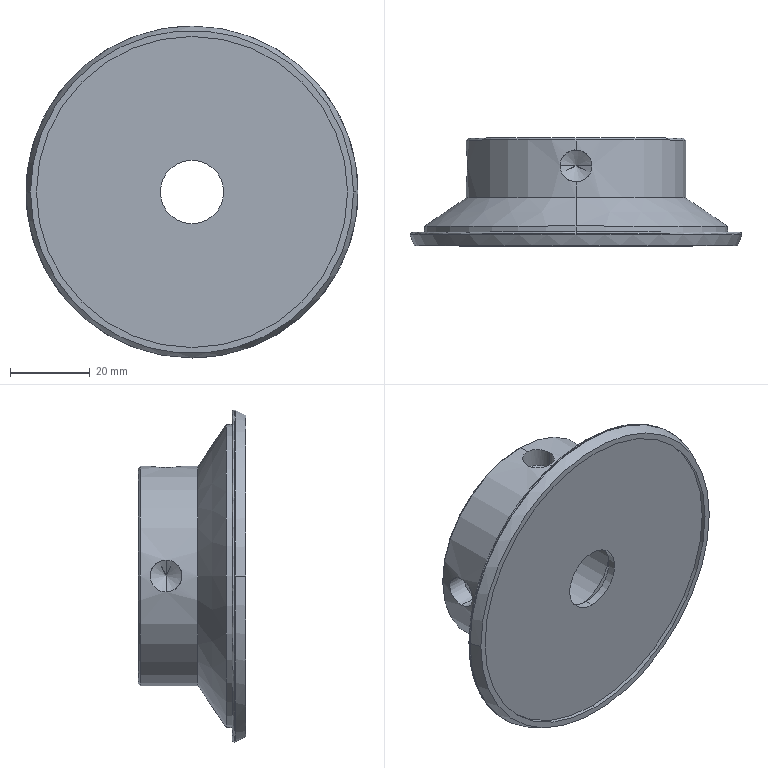Part | SolidWorks | features BaseBody 1 | 1 solid | 41 faces | box 83.227 x 27 x 83.227 mm | volume 68079 mm3 | cylinder 18 | cone 12 | plane 7 | spline 4 | commonest cylinder face diameters 8 x4 25 x4 15.9 x2 22 x2 55 x2 76 x2
STEP:
#1=CARTESIAN_POINT('',(0.,1.9,41.613));
#2=VERTEX_POINT('',#1);
#3=CARTESIAN_POINT('',(0.,1.9,-41.613));
#4=VERTEX_POINT('',#3);
#5=CARTESIAN_POINT('',(0.,1.9,0.));
#6=DIRECTION('',(0.,-1.,0.));
#7=DIRECTION('',(0.,0.,-1.));
#8=AXIS2_PLACEMENT_3D('',#5,#6,#7);
#9=CIRCLE('',#8,41.613);
#10=EDGE_CURVE('',#2,#4,#9,.T.);
#11=ORIENTED_EDGE('',*,*,#10,.F.);
#12=CARTESIAN_POINT('',(0.,2.4,41.113));
#13=VERTEX_POINT('',#12);
#14=CARTESIAN_POINT('',(0.,1.9,41.113));
#15=DIRECTION('',(-1.,0.,0.));
#16=DIRECTION('',(0.,0.,1.));
#17=AXIS2_PLACEMENT_3D('',#14,#15,#16);
#18=CIRCLE('',#17,0.5);
#19=EDGE_CURVE('',#2,#13,#18,.T.);
#20=ORIENTED_EDGE('',*,*,#19,.T.);
#21=CARTESIAN_POINT('',(0.,2.4,-41.113));
#22=VERTEX_POINT('',#21);
#23=CARTESIAN_POINT('',(0.,2.4,41.113));
#24=CARTESIAN_POINT('',(-82.227,2.4,41.113));
#25=CARTESIAN_POINT('',(-82.227,2.4,-41.113));
#26=CARTESIAN_POINT('',(0.,2.4,-41.113));
#27=(BOUNDED_CURVE()B_SPLINE_CURVE(3,(#23,#24,#25,#26),.UNSPECIFIED.,.F.,.F.)B_SPLINE_CURVE_WITH_KNOTS((4,4),(0.,1.),.UNSPECIFIED.)CURVE()GEOMETRIC_REPRESENTATION_ITEM()RATIONAL_B_SPLINE_CURVE((1.,0.3333,0.3333,1.))REPRESENTATION_ITEM(''));
#28=EDGE_CURVE('',#13,#22,#27,.T.);
#29=ORIENTED_EDGE('',*,*,#28,.T.);
#30=CARTESIAN_POINT('',(0.,1.9,-41.113));
#31=DIRECTION('',(1.,0.,0.));
#32=DIRECTION('',(0.,0.,-1.));
#33=AXIS2_PLACEMENT_3D('',#30,#31,#32);
#34=CIRCLE('',#33,0.5);
#35=EDGE_CURVE('',#4,#22,#34,.T.);
#36=ORIENTED_EDGE('',*,*,#35,.F.);
#37=EDGE_LOOP('',(#11,#20,#29,#36));
#38=FACE_OUTER_BOUND('',#37,.T.);
#39=CARTESIAN_POINT('',(0.,1.9,41.613));
#40=CARTESIAN_POINT('',(-83.227,1.9,41.613));
#41=CARTESIAN_POINT('',(-83.227,1.9,-41.613));
#42=CARTESIAN_POINT('',(0.,1.9,-41.613));
#43=CARTESIAN_POINT('',(0.,2.193,41.613));
#44=CARTESIAN_POINT('',(-83.227,2.193,41.613));
#45=CARTESIAN_POINT('',(-83.227,2.193,-41.613));
#46=CARTESIAN_POINT('',(0.,2.193,-41.613));
#47=CARTESIAN_POINT('',(0.,2.4,41.406));
#48=CARTESIAN_POINT('',(-82.813,2.4,41.406));
#49=CARTESIAN_POINT('',(-82.813,2.4,-41.406));
#50=CARTESIAN_POINT('',(0.,2.4,-41.406));
#51=CARTESIAN_POINT('',(0.,2.4,41.113));
#52=CARTESIAN_POINT('',(-82.227,2.4,41.113));
#53=CARTESIAN_POINT('',(-82.227,2.4,-41.113));
#54=CARTESIAN_POINT('',(0.,2.4,-41.113));
#55=(BOUNDED_SURFACE()B_SPLINE_SURFACE(3,3,((#39,#40,#41,#42),(#43,#44,#45,#46),(#47,#48,#49,#50),(#51,#52,#53,#54)),.UNSPECIFIED.,.F.,.F.,.F.)B_SPLINE_SURFACE_WITH_KNOTS((4,4),(4,4),(0.,1.),(0.,1.),.UNSPECIFIED.)GEOMETRIC_REPRESENTATION_ITEM()RATIONAL_B_SPLINE_SURFACE(((1.,0.3333,0.3333,1.),(0.8047,0.2682,0.2682,0.8047),(0.8047,0.2682,0.2682,0.8047),(1.,0.3333,0.3333,1.)))REPRESENTATION_ITEM('')SURFACE());
#56=ADVANCED_FACE('',(#38),#55,.T.);
#57=CARTESIAN_POINT('',(0.,1.715,41.578));
#58=VERTEX_POINT('',#57);
#59=CARTESIAN_POINT('',(-41.578,1.715,0.));
#60=VERTEX_POINT('',#59);
#61=CARTESIAN_POINT('',(0.,1.715,0.));
#62=DIRECTION('',(0.,-1.,0.));
#63=DIRECTION('',(0.,0.,1.));
#64=AXIS2_PLACEMENT_3D('',#61,#62,#63);
#65=CIRCLE('',#64,41.578);
#66=EDGE_CURVE('',#58,#60,#65,.T.);
#67=ORIENTED_EDGE('',*,*,#66,.F.);
#68=CARTESIAN_POINT('',(0.,1.9,41.113));
#69=DIRECTION('',(-1.,0.,0.));
#70=DIRECTION('',(0.,0.,1.));
#71=AXIS2_PLACEMENT_3D('',#68,#69,#70);
#72=CIRCLE('',#71,0.5);
#73=EDGE_CURVE('',#58,#2,#72,.T.);
#74=ORIENTED_EDGE('',*,*,#73,.T.);
#75=ORIENTED_EDGE('',*,*,#10,.T.);
#76=CARTESIAN_POINT('',(0.,1.715,-41.578));
#77=VERTEX_POINT('',#76);
#78=CARTESIAN_POINT('',(0.,1.9,-41.113));
#79=DIRECTION('',(1.,0.,0.));
#80=DIRECTION('',(0.,0.,-1.));
#81=AXIS2_PLACEMENT_3D('',#78,#79,#80);
#82=CIRCLE('',#81,0.5);
#83=EDGE_CURVE('',#77,#4,#82,.T.);
#84=ORIENTED_EDGE('',*,*,#83,.F.);
#85=CARTESIAN_POINT('',(0.,1.715,0.));
#86=DIRECTION('',(0.,-1.,0.));
#87=DIRECTION('',(0.,0.,1.));
#88=AXIS2_PLACEMENT_3D('',#85,#86,#87);
#89=CIRCLE('',#88,41.578);
#90=EDGE_CURVE('',#60,#77,#89,.T.);
#91=ORIENTED_EDGE('',*,*,#90,.F.);
#92=EDGE_LOOP('',(#67,#74,#75,#84,#91));
#93=FACE_OUTER_BOUND('',#92,.T.);
#94=CARTESIAN_POINT('',(0.,1.715,41.578));
#95=CARTESIAN_POINT('',(-83.156,1.715,41.578));
#96=CARTESIAN_POINT('',(-83.156,1.715,-41.578));
#97=CARTESIAN_POINT('',(0.,1.715,-41.578));
#98=CARTESIAN_POINT('',(0.,1.774,41.602));
#99=CARTESIAN_POINT('',(-83.203,1.774,41.602));
#100=CARTESIAN_POINT('',(-83.203,1.774,-41.602));
#101=CARTESIAN_POINT('',(0.,1.774,-41.602));
#102=CARTESIAN_POINT('',(0.,1.837,41.613));
#103=CARTESIAN_POINT('',(-83.227,1.837,41.613));
#104=CARTESIAN_POINT('',(-83.227,1.837,-41.613));
#105=CARTESIAN_POINT('',(0.,1.837,-41.613));
#106=CARTESIAN_POINT('',(0.,1.9,41.613));
#107=CARTESIAN_POINT('',(-83.227,1.9,41.613));
#108=CARTESIAN_POINT('',(-83.227,1.9,-41.613));
#109=CARTESIAN_POINT('',(0.,1.9,-41.613));
#110=(BOUNDED_SURFACE()B_SPLINE_SURFACE(3,3,((#94,#95,#96,#97),(#98,#99,#100,#101),(#102,#103,#104,#105),(#106,#107,#108,#109)),.UNSPECIFIED.,.F.,.F.,.F.)B_SPLINE_SURFACE_WITH_KNOTS((4,4),(4,4),(0.,1.),(0.,1.),.UNSPECIFIED.)GEOMETRIC_REPRESENTATION_ITEM()RATIONAL_B_SPLINE_SURFACE(((1.,0.3333,0.3333,1.),(0.9881,0.3294,0.3294,0.9881),(0.9881,0.3294,0.3294,0.9881),(1.,0.3333,0.3333,1.)))REPRESENTATION_ITEM('')SURFACE());
#111=ADVANCED_FACE('',(#93),#110,.T.);
#112=CARTESIAN_POINT('',(0.,0.,-39.));
#113=VERTEX_POINT('',#112);
#114=CARTESIAN_POINT('',(0.,0.,39.));
#115=VERTEX_POINT('',#114);
#116=CARTESIAN_POINT('',(0.,0.,0.));
#117=DIRECTION('',(0.,1.,0.));
#118=DIRECTION('',(0.,0.,-1.));
#119=AXIS2_PLACEMENT_3D('',#116,#117,#118);
#120=CIRCLE('',#119,39.);
#121=EDGE_CURVE('',#113,#115,#120,.T.);
#122=ORIENTED_EDGE('',*,*,#121,.T.);
#123=CARTESIAN_POINT('',(0.,-1.,39.));
#124=VERTEX_POINT('',#123);
#125=CARTESIAN_POINT('',(0.,0.,39.));
#126=DIRECTION('',(0.,-1.,0.));
#127=VECTOR('',#126,1000.);
#128=LINE('',#125,#127);
#129=EDGE_CURVE('',#115,#124,#128,.T.);
#130=ORIENTED_EDGE('',*,*,#129,.T.);
#131=CARTESIAN_POINT('',(0.,-1.,-39.));
#132=VERTEX_POINT('',#131);
#133=CARTESIAN_POINT('',(0.,-1.,0.));
#134=DIRECTION('',(0.,1.,0.));
#135=DIRECTION('',(0.,0.,-1.));
#136=AXIS2_PLACEMENT_3D('',#133,#134,#135);
#137=CIRCLE('',#136,39.);
#138=EDGE_CURVE('',#132,#124,#137,.T.);
#139=ORIENTED_EDGE('',*,*,#138,.F.);
#140=CARTESIAN_POINT('',(0.,0.,-39.));
#141=DIRECTION('',(0.,-1.,0.));
#142=VECTOR('',#141,1000.);
#143=LINE('',#140,#142);
#144=EDGE_CURVE('',#113,#132,#143,.T.);
#145=ORIENTED_EDGE('',*,*,#144,.F.);
#146=EDGE_LOOP('',(#122,#130,#139,#145));
#147=FACE_OUTER_BOUND('',#146,.T.);
#148=CARTESIAN_POINT('',(0.,0.,0.));
#149=DIRECTION('',(0.,-1.,0.));
#150=DIRECTION('',(0.,0.,-1.));
#151=AXIS2_PLACEMENT_3D('',#148,#149,#150);
#152=CYLINDRICAL_SURFACE('',#151,39.);
#153=ADVANCED_FACE('',(#147),#152,.F.);
#154=CARTESIAN_POINT('',(0.,2.,7.95));
#155=VERTEX_POINT('',#154);
#156=CARTESIAN_POINT('',(0.,2.,-7.95));
#157=VERTEX_POINT('',#156);
#158=CARTESIAN_POINT('',(0.,2.,0.));
#159=DIRECTION('',(0.,-1.,0.));
#160=DIRECTION('',(0.,0.,-1.));
#161=AXIS2_PLACEMENT_3D('',#158,#159,#160);
#162=CIRCLE('',#161,7.95);
#163=EDGE_CURVE('',#155,#157,#162,.T.);
#164=ORIENTED_EDGE('',*,*,#163,.F.);
#165=CARTESIAN_POINT('',(0.,0.,7.95));
#166=VERTEX_POINT('',#165);
#167=CARTESIAN_POINT('',(0.,0.,7.95));
#168=DIRECTION('',(0.,-1.,0.));
#169=VECTOR('',#168,1000.);
#170=LINE('',#167,#169);
#171=EDGE_CURVE('',#155,#166,#170,.T.);
#172=ORIENTED_EDGE('',*,*,#171,.T.);
#173=CARTESIAN_POINT('',(0.,0.,-7.95));
#174=VERTEX_POINT('',#173);
#175=CARTESIAN_POINT('',(0.,0.,0.));
#176=DIRECTION('',(0.,-1.,0.));
#177=DIRECTION('',(0.,0.,-1.));
#178=AXIS2_PLACEMENT_3D('',#175,#176,#177);
#179=CIRCLE('',#178,7.95);
#180=EDGE_CURVE('',#166,#174,#179,.T.);
#181=ORIENTED_EDGE('',*,*,#180,.T.);
#182=CARTESIAN_POINT('',(0.,0.,-7.95));
#183=DIRECTION('',(0.,-1.,0.));
#184=VECTOR('',#183,1000.);
#185=LINE('',#182,#184);
#186=EDGE_CURVE('',#157,#174,#185,.T.);
#187=ORIENTED_EDGE('',*,*,#186,.F.);
#188=EDGE_LOOP('',(#164,#172,#181,#187));
#189=FACE_OUTER_BOUND('',#188,.T.);
#190=CARTESIAN_POINT('',(0.,0.,0.));
#191=DIRECTION('',(0.,-1.,0.));
#192=DIRECTION('',(0.,0.,-1.));
#193=AXIS2_PLACEMENT_3D('',#190,#191,#192);
#194=CYLINDRICAL_SURFACE('',#193,7.95);
#195=ADVANCED_FACE('',(#189),#194,.F.);
#196=CARTESIAN_POINT('',(-40.5,-1.,0.));
#197=VERTEX_POINT('',#196);
#198=CARTESIAN_POINT('',(40.5,-1.,0.));
#199=VERTEX_POINT('',#198);
#200=CARTESIAN_POINT('',(0.,-1.,0.));
#201=DIRECTION('',(0.,1.,0.));
#202=DIRECTION('',(-1.,0.,0.));
#203=AXIS2_PLACEMENT_3D('',#200,#201,#202);
#204=CIRCLE('',#203,40.5);
#205=EDGE_CURVE('',#197,#199,#204,.T.);
#206=ORIENTED_EDGE('',*,*,#205,.T.);
#207=CARTESIAN_POINT('',(41.578,1.715,0.));
#208=VERTEX_POINT('',#207);
#209=CARTESIAN_POINT('',(41.578,1.715,0.));
#210=DIRECTION('',(0.369,0.9294,0.));
#211=VECTOR('',#210,1000.);
#212=LINE('',#209,#211);
#213=EDGE_CURVE('',#199,#208,#212,.T.);
#214=ORIENTED_EDGE('',*,*,#213,.T.);
#215=CARTESIAN_POINT('',(0.,1.715,0.));
#216=DIRECTION('',(0.,-1.,0.));
#217=DIRECTION('',(0.,0.,1.));
#218=AXIS2_PLACEMENT_3D('',#215,#216,#217);
#219=CIRCLE('',#218,41.578);
#220=EDGE_CURVE('',#208,#58,#219,.T.);
#221=ORIENTED_EDGE('',*,*,#220,.T.);
#222=ORIENTED_EDGE('',*,*,#66,.T.);
#223=CARTESIAN_POINT('',(-41.578,1.715,0.));
#224=DIRECTION('',(-0.369,0.9294,0.));
#225=VECTOR('',#224,1000.);
#226=LINE('',#223,#225);
#227=EDGE_CURVE('',#197,#60,#226,.T.);
#228=ORIENTED_EDGE('',*,*,#227,.F.);
#229=EDGE_LOOP('',(#206,#214,#221,#222,#228));
#230=FACE_OUTER_BOUND('',#229,.T.);
#231=CARTESIAN_POINT('',(0.,1.715,0.));
#232=DIRECTION('',(0.,1.,0.));
#233=DIRECTION('',(-1.,0.,0.));
#234=AXIS2_PLACEMENT_3D('',#231,#232,#233);
#235=CONICAL_SURFACE('',#234,41.578,0.378);
#236=ADVANCED_FACE('',(#230),#235,.T.);
#237=CARTESIAN_POINT('',(0.,5.,12.5));
#238=VERTEX_POINT('',#237);
#239=CARTESIAN_POINT('',(0.,5.,-12.5));
#240=VERTEX_POINT('',#239);
#241=CARTESIAN_POINT('',(0.,5.,0.));
#242=DIRECTION('',(0.,-1.,0.));
#243=DIRECTION('',(0.,0.,-1.));
#244=AXIS2_PLACEMENT_3D('',#241,#242,#243);
#245=CIRCLE('',#244,12.5);
#246=EDGE_CURVE('',#238,#240,#245,.T.);
#247=ORIENTED_EDGE('',*,*,#246,.F.);
#248=CARTESIAN_POINT('',(0.,2.,12.5));
#249=VERTEX_POINT('',#248);
#250=CARTESIAN_POINT('',(0.,0.,12.5));
#251=DIRECTION('',(0.,-1.,0.));
#252=VECTOR('',#251,1000.);
#253=LINE('',#250,#252);
#254=EDGE_CURVE('',#238,#249,#253,.T.);
#255=ORIENTED_EDGE('',*,*,#254,.T.);
#256=CARTESIAN_POINT('',(0.,2.,-12.5));
#257=VERTEX_POINT('',#256);
#258=CARTESIAN_POINT('',(0.,2.,0.));
#259=DIRECTION('',(0.,-1.,0.));
#260=DIRECTION('',(0.,0.,-1.));
#261=AXIS2_PLACEMENT_3D('',#258,#259,#260);
#262=CIRCLE('',#261,12.5);
#263=EDGE_CURVE('',#249,#257,#262,.T.);
#264=ORIENTED_EDGE('',*,*,#263,.T.);
#265=CARTESIAN_POINT('',(0.,0.,-12.5));
#266=DIRECTION('',(0.,-1.,0.));
#267=VECTOR('',#266,1000.);
#268=LINE('',#265,#267);
#269=EDGE_CURVE('',#240,#257,#268,.T.);
#270=ORIENTED_EDGE('',*,*,#269,.F.);
#271=EDGE_LOOP('',(#247,#255,#264,#270));
#272=FACE_OUTER_BOUND('',#271,.T.);
#273=CARTESIAN_POINT('',(0.,0.,0.));
#274=DIRECTION('',(0.,-1.,0.));
#275=DIRECTION('',(0.,0.,-1.));
#276=AXIS2_PLACEMENT_3D('',#273,#274,#275);
#277=CYLINDRICAL_SURFACE('',#276,12.5);
#278=ADVANCED_FACE('',(#272),#277,.F.);
#279=ORIENTED_EDGE('',*,*,#73,.F.);
#280=ORIENTED_EDGE('',*,*,#220,.F.);
#281=CARTESIAN_POINT('',(0.,1.715,0.));
#282=DIRECTION('',(0.,-1.,0.));
#283=DIRECTION('',(0.,0.,1.));
#284=AXIS2_PLACEMENT_3D('',#281,#282,#283);
#285=CIRCLE('',#284,41.578);
#286=EDGE_CURVE('',#77,#208,#285,.T.);
#287=ORIENTED_EDGE('',*,*,#286,.F.);
#288=ORIENTED_EDGE('',*,*,#83,.T.);
#289=CARTESIAN_POINT('',(0.,1.9,0.));
#290=DIRECTION('',(0.,-1.,0.));
#291=DIRECTION('',(0.,0.,-1.));
#292=AXIS2_PLACEMENT_3D('',#289,#290,#291);
#293=CIRCLE('',#292,41.613);
#294=EDGE_CURVE('',#4,#2,#293,.T.);
#295=ORIENTED_EDGE('',*,*,#294,.T.);
#296=EDGE_LOOP('',(#279,#280,#287,#288,#295));
#297=FACE_OUTER_BOUND('',#296,.T.);
#298=CARTESIAN_POINT('',(0.,1.715,-41.578));
#299=CARTESIAN_POINT('',(83.156,1.715,-41.578));
#300=CARTESIAN_POINT('',(83.156,1.715,41.578));
#301=CARTESIAN_POINT('',(0.,1.715,41.578));
#302=CARTESIAN_POINT('',(0.,1.774,-41.602));
#303=CARTESIAN_POINT('',(83.203,1.774,-41.602));
#304=CARTESIAN_POINT('',(83.203,1.774,41.602));
#305=CARTESIAN_POINT('',(0.,1.774,41.602));
#306=CARTESIAN_POINT('',(0.,1.837,-41.613));
#307=CARTESIAN_POINT('',(83.227,1.837,-41.613));
#308=CARTESIAN_POINT('',(83.227,1.837,41.613));
#309=CARTESIAN_POINT('',(0.,1.837,41.613));
#310=CARTESIAN_POINT('',(0.,1.9,-41.613));
#311=CARTESIAN_POINT('',(83.227,1.9,-41.613));
#312=CARTESIAN_POINT('',(83.227,1.9,41.613));
#313=CARTESIAN_POINT('',(0.,1.9,41.613));
#314=(BOUNDED_SURFACE()B_SPLINE_SURFACE(3,3,((#298,#299,#300,#301),(#302,#303,#304,#305),(#306,#307,#308,#309),(#310,#311,#312,#313)),.UNSPECIFIED.,.F.,.F.,.F.)B_SPLINE_SURFACE_WITH_KNOTS((4,4),(4,4),(0.,1.),(0.,1.),.UNSPECIFIED.)GEOMETRIC_REPRESENTATION_ITEM()RATIONAL_B_SPLINE_SURFACE(((1.,0.3333,0.3333,1.),(0.9881,0.3294,0.3294,0.9881),(0.9881,0.3294,0.3294,0.9881),(1.,0.3333,0.3333,1.)))REPRESENTATION_ITEM('')SURFACE());
#315=ADVANCED_FACE('',(#297),#314,.T.);
#316=CARTESIAN_POINT('',(0.,14.,11.));
#317=VERTEX_POINT('',#316);
#318=CARTESIAN_POINT('',(0.,14.,-11.));
#319=VERTEX_POINT('',#318);
#320=CARTESIAN_POINT('',(0.,14.,0.));
#321=DIRECTION('',(0.,-1.,0.));
#322=DIRECTION('',(0.,0.,-1.));
#323=AXIS2_PLACEMENT_3D('',#320,#321,#322);
#324=CIRCLE('',#323,11.);
#325=EDGE_CURVE('',#317,#319,#324,.T.);
#326=ORIENTED_EDGE('',*,*,#325,.F.);
#327=CARTESIAN_POINT('',(0.,5.,11.));
#328=VERTEX_POINT('',#327);
#329=CARTESIAN_POINT('',(0.,0.,11.));
#330=DIRECTION('',(0.,-1.,0.));
#331=VECTOR('',#330,1000.);
#332=LINE('',#329,#331);
#333=EDGE_CURVE('',#317,#328,#332,.T.);
#334=ORIENTED_EDGE('',*,*,#333,.T.);
#335=CARTESIAN_POINT('',(0.,5.,-11.));
#336=VERTEX_POINT('',#335);
#337=CARTESIAN_POINT('',(0.,5.,0.));
#338=DIRECTION('',(0.,-1.,0.));
#339=DIRECTION('',(0.,0.,-1.));
#340=AXIS2_PLACEMENT_3D('',#337,#338,#339);
#341=CIRCLE('',#340,11.);
#342=EDGE_CURVE('',#328,#336,#341,.T.);
#343=ORIENTED_EDGE('',*,*,#342,.T.);
#344=CARTESIAN_POINT('',(0.,0.,-11.));
#345=DIRECTION('',(0.,-1.,0.));
#346=VECTOR('',#345,1000.);
#347=LINE('',#344,#346);
#348=EDGE_CURVE('',#319,#336,#347,.T.);
#349=ORIENTED_EDGE('',*,*,#348,.F.);
#350=EDGE_LOOP('',(#326,#334,#343,#349));
#351=FACE_OUTER_BOUND('',#350,.T.);
#352=CARTESIAN_POINT('',(0.,0.,0.));
#353=DIRECTION('',(0.,-1.,0.));
#354=DIRECTION('',(0.,0.,-1.));
#355=AXIS2_PLACEMENT_3D('',#352,#353,#354);
#356=CYLINDRICAL_SURFACE('',#355,11.);
#357=ADVANCED_FACE('',(#351),#356,.F.);
#358=CARTESIAN_POINT('',(0.,3.9,-38.));
#359=VERTEX_POINT('',#358);
#360=CARTESIAN_POINT('',(0.,3.9,38.));
#361=VERTEX_POINT('',#360);
#362=CARTESIAN_POINT('',(0.,3.9,0.));
#363=DIRECTION('',(0.,-1.,0.));
#364=DIRECTION('',(0.,0.,-1.));
#365=AXIS2_PLACEMENT_3D('',#362,#363,#364);
#366=CIRCLE('',#365,38.);
#367=EDGE_CURVE('',#359,#361,#366,.T.);
#368=ORIENTED_EDGE('',*,*,#367,.T.);
#369=CARTESIAN_POINT('',(0.,2.4,38.));
#370=VERTEX_POINT('',#369);
#371=CARTESIAN_POINT('',(0.,0.,38.));
#372=DIRECTION('',(0.,-1.,0.));
#373=VECTOR('',#372,1000.);
#374=LINE('',#371,#373);
#375=EDGE_CURVE('',#361,#370,#374,.T.);
#376=ORIENTED_EDGE('',*,*,#375,.T.);
#377=CARTESIAN_POINT('',(0.,2.4,-38.));
#378=VERTEX_POINT('',#377);
#379=CARTESIAN_POINT('',(0.,2.4,0.));
#380=DIRECTION('',(0.,1.,0.));
#381=DIRECTION('',(0.,0.,-1.));
#382=AXIS2_PLACEMENT_3D('',#379,#380,#381);
#383=CIRCLE('',#382,38.);
#384=EDGE_CURVE('',#370,#378,#383,.T.);
#385=ORIENTED_EDGE('',*,*,#384,.T.);
#386=CARTESIAN_POINT('',(0.,0.,-38.));
#387=DIRECTION('',(0.,-1.,0.));
#388=VECTOR('',#387,1000.);
#389=LINE('',#386,#388);
#390=EDGE_CURVE('',#359,#378,#389,.T.);
#391=ORIENTED_EDGE('',*,*,#390,.F.);
#392=EDGE_LOOP('',(#368,#376,#385,#391));
#393=FACE_OUTER_BOUND('',#392,.T.);
#394=CARTESIAN_POINT('',(0.,0.,0.));
#395=DIRECTION('',(0.,-1.,0.));
#396=DIRECTION('',(0.,0.,-1.));
#397=AXIS2_PLACEMENT_3D('',#394,#395,#396);
#398=CYLINDRICAL_SURFACE('',#397,38.);
#399=ADVANCED_FACE('',(#393),#398,.T.);
#400=CARTESIAN_POINT('',(0.,11.,-27.5));
#401=VERTEX_POINT('',#400);
#402=CARTESIAN_POINT('',(0.,11.,27.5));
#403=VERTEX_POINT('',#402);
#404=CARTESIAN_POINT('',(0.,11.,0.));
#405=DIRECTION('',(0.,-1.,0.));
#406=DIRECTION('',(0.,0.,-1.));
#407=AXIS2_PLACEMENT_3D('',#404,#405,#406);
#408=CIRCLE('',#407,27.5);
#409=EDGE_CURVE('',#401,#403,#408,.T.);
#410=ORIENTED_EDGE('',*,*,#409,.T.);
#411=CARTESIAN_POINT('',(0.,3.9,38.));
#412=DIRECTION('',(0.,-0.5602,0.8284));
#413=VECTOR('',#412,1000.);
#414=LINE('',#411,#413);
#415=EDGE_CURVE('',#403,#361,#414,.T.);
#416=ORIENTED_EDGE('',*,*,#415,.T.);
#417=ORIENTED_EDGE('',*,*,#367,.F.);
#418=CARTESIAN_POINT('',(0.,3.9,-38.));
#419=DIRECTION('',(0.,-0.5602,-0.8284));
#420=VECTOR('',#419,1000.);
#421=LINE('',#418,#420);
#422=EDGE_CURVE('',#401,#359,#421,.T.);
#423=ORIENTED_EDGE('',*,*,#422,.F.);
#424=EDGE_LOOP('',(#410,#416,#417,#423));
#425=FACE_OUTER_BOUND('',#424,.T.);
#426=CARTESIAN_POINT('',(0.,3.9,0.));
#427=DIRECTION('',(0.,-1.,0.));
#428=DIRECTION('',(0.,0.,-1.));
#429=AXIS2_PLACEMENT_3D('',#426,#427,#428);
#430=CONICAL_SURFACE('',#429,38.,0.9762);
#431=ADVANCED_FACE('',(#425),#430,.T.);
#432=CARTESIAN_POINT('',(0.,25.5,12.5));
#433=VERTEX_POINT('',#432);
#434=CARTESIAN_POINT('',(0.,25.5,-12.5));
#435=VERTEX_POINT('',#434);
#436=CARTESIAN_POINT('',(0.,25.5,0.));
#437=DIRECTION('',(0.,-1.,0.));
#438=DIRECTION('',(0.,0.,-1.));
#439=AXIS2_PLACEMENT_3D('',#436,#437,#438);
#440=CIRCLE('',#439,12.5);
#441=EDGE_CURVE('',#433,#435,#440,.T.);
#442=ORIENTED_EDGE('',*,*,#441,.F.);
#443=CARTESIAN_POINT('',(0.,14.,12.5));
#444=VERTEX_POINT('',#443);
#445=CARTESIAN_POINT('',(0.,0.,12.5));
#446=DIRECTION('',(0.,-1.,0.));
#447=VECTOR('',#446,1000.);
#448=LINE('',#445,#447);
#449=EDGE_CURVE('',#433,#444,#448,.T.);
#450=ORIENTED_EDGE('',*,*,#449,.T.);
#451=CARTESIAN_POINT('',(0.,14.,-12.5));
#452=VERTEX_POINT('',#451);
#453=CARTESIAN_POINT('',(0.,14.,0.));
#454=DIRECTION('',(0.,-1.,0.));
#455=DIRECTION('',(0.,0.,-1.));
#456=AXIS2_PLACEMENT_3D('',#453,#454,#455);
#457=CIRCLE('',#456,12.5);
#458=EDGE_CURVE('',#444,#452,#457,.T.);
#459=ORIENTED_EDGE('',*,*,#458,.T.);
#460=CARTESIAN_POINT('',(0.,0.,-12.5));
#461=DIRECTION('',(0.,-1.,0.));
#462=VECTOR('',#461,1000.);
#463=LINE('',#460,#462);
#464=EDGE_CURVE('',#435,#452,#463,.T.);
#465=ORIENTED_EDGE('',*,*,#464,.F.);
#466=EDGE_LOOP('',(#442,#450,#459,#465));
#467=FACE_OUTER_BOUND('',#466,.T.);
#468=CARTESIAN_POINT('',(0.,0.,0.));
#469=DIRECTION('',(0.,-1.,0.));
#470=DIRECTION('',(0.,0.,-1.));
#471=AXIS2_PLACEMENT_3D('',#468,#469,#470);
#472=CYLINDRICAL_SURFACE('',#471,12.5);
#473=ADVANCED_FACE('',(#467),#472,.F.);
#474=CARTESIAN_POINT('',(27.5,25.5,0.));
#475=VERTEX_POINT('',#474);
#476=CARTESIAN_POINT('',(0.,25.5,27.5));
#477=VERTEX_POINT('',#476);
#478=CARTESIAN_POINT('',(0.,25.5,0.));
#479=DIRECTION('',(0.,-1.,0.));
#480=DIRECTION('',(0.,0.,-1.));
#481=AXIS2_PLACEMENT_3D('',#478,#479,#480);
#482=CIRCLE('',#481,27.5);
#483=EDGE_CURVE('',#475,#477,#482,.T.);
#484=ORIENTED_EDGE('',*,*,#483,.T.);
#485=CARTESIAN_POINT('',(0.,23.,27.5));
#486=VERTEX_POINT('',#485);
#487=CARTESIAN_POINT('',(0.,0.,27.5));
#488=DIRECTION('',(0.,-1.,0.));
#489=VECTOR('',#488,1000.);
#490=LINE('',#487,#489);
#491=EDGE_CURVE('',#477,#486,#490,.T.);
#492=ORIENTED_EDGE('',*,*,#491,.T.);
#493=CARTESIAN_POINT('',(4.,19.,27.208));
#494=VERTEX_POINT('',#493);
#495=CARTESIAN_POINT('',(0.,23.,27.5));
#496=CARTESIAN_POINT('',(0.2645,23.,27.5));
#497=CARTESIAN_POINT('',(0.5245,22.974,27.496));
#498=CARTESIAN_POINT('',(1.036,22.872,27.482));
#499=CARTESIAN_POINT('',(1.29,22.795,27.471));
#500=CARTESIAN_POINT('',(1.774,22.595,27.444));
#501=CARTESIAN_POINT('',(2.004,22.472,27.428));
#502=CARTESIAN_POINT('',(2.438,22.182,27.393));
#503=CARTESIAN_POINT('',(2.643,22.013,27.373));
#504=CARTESIAN_POINT('',(3.012,21.645,27.335));
#505=CARTESIAN_POINT('',(3.177,21.444,27.316));
#506=CARTESIAN_POINT('',(3.47,21.008,27.281));
#507=CARTESIAN_POINT('',(3.594,20.776,27.264));
#508=CARTESIAN_POINT('',(3.794,20.295,27.237));
#509=CARTESIAN_POINT('',(3.871,20.043,27.226));
#510=CARTESIAN_POINT('',(3.974,19.526,27.211));
#511=CARTESIAN_POINT('',(4.,19.264,27.208));
#512=CARTESIAN_POINT('',(4.,19.,27.208));
#513=B_SPLINE_CURVE_WITH_KNOTS('',3,(#495,#496,#497,#498,#499,#500,#501,#502,#503,#504,#505,#506,#507,#508,#509,#510,#511,#512),.UNSPECIFIED.,.F.,.F.,(4,2,2,2,2,2,2,2,4),(-0.006257,-0.005475,-0.004693,-0.003911,-0.003128,-0.002346,-0.001564,-0.0007821,0.),.UNSPECIFIED.);
#514=EDGE_CURVE('',#486,#494,#513,.T.);
#515=ORIENTED_EDGE('',*,*,#514,.T.);
#516=CARTESIAN_POINT('',(0.,15.,27.5));
#517=VERTEX_POINT('',#516);
#518=CARTESIAN_POINT('',(4.,19.,27.208));
#519=CARTESIAN_POINT('',(4.,18.736,27.208));
#520=CARTESIAN_POINT('',(3.974,18.476,27.211));
#521=CARTESIAN_POINT('',(3.872,17.964,27.226));
#522=CARTESIAN_POINT('',(3.795,17.71,27.237));
#523=CARTESIAN_POINT('',(3.595,17.226,27.264));
#524=CARTESIAN_POINT('',(3.472,16.996,27.28));
#525=CARTESIAN_POINT('',(3.182,16.562,27.316));
#526=CARTESIAN_POINT('',(3.013,16.357,27.335));
#527=CARTESIAN_POINT('',(2.645,15.988,27.373));
#528=CARTESIAN_POINT('',(2.444,15.823,27.392));
#529=CARTESIAN_POINT('',(2.008,15.53,27.427));
#530=CARTESIAN_POINT('',(1.776,15.406,27.444));
#531=CARTESIAN_POINT('',(1.295,15.206,27.471));
#532=CARTESIAN_POINT('',(1.043,15.129,27.481));
#533=CARTESIAN_POINT('',(0.526,15.026,27.496));
#534=CARTESIAN_POINT('',(0.2645,15.,27.5));
#535=CARTESIAN_POINT('',(0.,15.,27.5));
#536=B_SPLINE_CURVE_WITH_KNOTS('',3,(#518,#519,#520,#521,#522,#523,#524,#525,#526,#527,#528,#529,#530,#531,#532,#533,#534,#535),.UNSPECIFIED.,.F.,.F.,(4,2,2,2,2,2,2,2,4),(0.,0.0007821,0.001564,0.002346,0.003128,0.003911,0.004693,0.005475,0.006257),.UNSPECIFIED.);
#537=EDGE_CURVE('',#494,#517,#536,.T.);
#538=ORIENTED_EDGE('',*,*,#537,.T.);
#539=CARTESIAN_POINT('',(0.,0.,27.5));
#540=DIRECTION('',(0.,-1.,0.));
#541=VECTOR('',#540,1000.);
#542=LINE('',#539,#541);
#543=EDGE_CURVE('',#517,#403,#542,.T.);
#544=ORIENTED_EDGE('',*,*,#543,.T.);
#545=ORIENTED_EDGE('',*,*,#409,.F.);
#546=CARTESIAN_POINT('',(0.,25.5,-27.5));
#547=VERTEX_POINT('',#546);
#548=CARTESIAN_POINT('',(0.,0.,-27.5));
#549=DIRECTION('',(0.,-1.,0.));
#550=VECTOR('',#549,1000.);
#551=LINE('',#548,#550);
#552=EDGE_CURVE('',#547,#401,#551,.T.);
#553=ORIENTED_EDGE('',*,*,#552,.F.);
#554=CARTESIAN_POINT('',(0.,25.5,0.));
#555=DIRECTION('',(0.,-1.,0.));
#556=DIRECTION('',(0.,0.,-1.));
#557=AXIS2_PLACEMENT_3D('',#554,#555,#556);
#558=CIRCLE('',#557,27.5);
#559=EDGE_CURVE('',#547,#475,#558,.T.);
#560=ORIENTED_EDGE('',*,*,#559,.T.);
#561=EDGE_LOOP('',(#484,#492,#515,#538,#544,#545,#553,#560));
#562=FACE_OUTER_BOUND('',#561,.T.);
#563=CARTESIAN_POINT('',(0.,0.,0.));
#564=DIRECTION('',(0.,-1.,0.));
#565=DIRECTION('',(0.,0.,-1.));
#566=AXIS2_PLACEMENT_3D('',#563,#564,#565);
#567=CYLINDRICAL_SURFACE('',#566,27.5);
#568=ADVANCED_FACE('',(#562),#567,.T.);
#569=ORIENTED_EDGE('',*,*,#441,.T.);
#570=CARTESIAN_POINT('',(0.,26.,-13.));
#571=VERTEX_POINT('',#570);
#572=CARTESIAN_POINT('',(0.,26.,-13.));
#573=DIRECTION('',(0.,0.7071,-0.7071));
#574=VECTOR('',#573,1000.);
#575=LINE('',#572,#574);
#576=EDGE_CURVE('',#435,#571,#575,.T.);
#577=ORIENTED_EDGE('',*,*,#576,.T.);
#578=CARTESIAN_POINT('',(0.,26.,13.));
#579=VERTEX_POINT('',#578);
#580=CARTESIAN_POINT('',(0.,26.,0.));
#581=DIRECTION('',(0.,-1.,0.));
#582=DIRECTION('',(0.,0.,1.));
#583=AXIS2_PLACEMENT_3D('',#580,#581,#582);
#584=CIRCLE('',#583,13.);
#585=EDGE_CURVE('',#579,#571,#584,.T.);
#586=ORIENTED_EDGE('',*,*,#585,.F.);
#587=CARTESIAN_POINT('',(0.,26.,13.));
#588=DIRECTION('',(0.,0.7071,0.7071));
#589=VECTOR('',#588,1000.);
#590=LINE('',#587,#589);
#591=EDGE_CURVE('',#433,#579,#590,.T.);
#592=ORIENTED_EDGE('',*,*,#591,.F.);
#593=EDGE_LOOP('',(#569,#577,#586,#592));
#594=FACE_OUTER_BOUND('',#593,.T.);
#595=CARTESIAN_POINT('',(0.,26.,0.));
#596=DIRECTION('',(0.,1.,0.));
#597=DIRECTION('',(0.,0.,1.));
#598=AXIS2_PLACEMENT_3D('',#595,#596,#597);
#599=CONICAL_SURFACE('',#598,13.,0.7854);
#600=ADVANCED_FACE('',(#594),#599,.F.);
#601=CARTESIAN_POINT('',(-4.,19.,22.5));
#602=VERTEX_POINT('',#601);
#603=CARTESIAN_POINT('',(4.,19.,22.5));
#604=VERTEX_POINT('',#603);
#605=CARTESIAN_POINT('',(0.,19.,22.5));
#606=DIRECTION('',(0.,0.,1.));
#607=DIRECTION('',(1.,0.,0.));
#608=AXIS2_PLACEMENT_3D('',#605,#606,#607);
#609=CIRCLE('',#608,4.);
#610=EDGE_CURVE('',#602,#604,#609,.T.);
#611=ORIENTED_EDGE('',*,*,#610,.F.);
#612=CARTESIAN_POINT('',(-4.,19.,27.208));
#613=VERTEX_POINT('',#612);
#614=CARTESIAN_POINT('',(-4.,19.,27.5));
#615=DIRECTION('',(0.,0.,1.));
#616=VECTOR('',#615,1000.);
#617=LINE('',#614,#616);
#618=EDGE_CURVE('',#602,#613,#617,.T.);
#619=ORIENTED_EDGE('',*,*,#618,.T.);
#620=CARTESIAN_POINT('',(0.,15.,27.5));
#621=CARTESIAN_POINT('',(-0.2645,15.,27.5));
#622=CARTESIAN_POINT('',(-0.5245,15.026,27.496));
#623=CARTESIAN_POINT('',(-1.036,15.128,27.482));
#624=CARTESIAN_POINT('',(-1.29,15.205,27.471));
#625=CARTESIAN_POINT('',(-1.774,15.405,27.444));
#626=CARTESIAN_POINT('',(-2.004,15.528,27.428));
#627=CARTESIAN_POINT('',(-2.438,15.818,27.393));
#628=CARTESIAN_POINT('',(-2.643,15.987,27.373));
#629=CARTESIAN_POINT('',(-3.012,16.355,27.335));
#630=CARTESIAN_POINT('',(-3.177,16.556,27.316));
#631=CARTESIAN_POINT('',(-3.47,16.992,27.281));
#632=CARTESIAN_POINT('',(-3.594,17.224,27.264));
#633=CARTESIAN_POINT('',(-3.794,17.705,27.237));
#634=CARTESIAN_POINT('',(-3.871,17.957,27.226));
#635=CARTESIAN_POINT('',(-3.974,18.474,27.211));
#636=CARTESIAN_POINT('',(-4.,18.736,27.208));
#637=CARTESIAN_POINT('',(-4.,19.,27.208));
#638=B_SPLINE_CURVE_WITH_KNOTS('',3,(#620,#621,#622,#623,#624,#625,#626,#627,#628,#629,#630,#631,#632,#633,#634,#635,#636,#637),.UNSPECIFIED.,.F.,.F.,(4,2,2,2,2,2,2,2,4),(0.006257,0.007039,0.007821,0.008603,0.009385,0.01017,0.01095,0.01173,0.01251),.UNSPECIFIED.);
#639=EDGE_CURVE('',#517,#613,#638,.T.);
#640=ORIENTED_EDGE('',*,*,#639,.F.);
#641=ORIENTED_EDGE('',*,*,#537,.F.);
#642=CARTESIAN_POINT('',(4.,19.,27.5));
#643=DIRECTION('',(0.,0.,1.));
#644=VECTOR('',#643,1000.);
#645=LINE('',#642,#644);
#646=EDGE_CURVE('',#604,#494,#645,.T.);
#647=ORIENTED_EDGE('',*,*,#646,.F.);
#648=EDGE_LOOP('',(#611,#619,#640,#641,#647));
#649=FACE_OUTER_BOUND('',#648,.T.);
#650=CARTESIAN_POINT('',(0.,19.,27.5));
#651=DIRECTION('',(0.,0.,1.));
#652=DIRECTION('',(1.,0.,0.));
#653=AXIS2_PLACEMENT_3D('',#650,#651,#652);
#654=CYLINDRICAL_SURFACE('',#653,4.);
#655=ADVANCED_FACE('',(#649),#654,.F.);
#656=CARTESIAN_POINT('',(27.,26.,0.));
#657=VERTEX_POINT('',#656);
#658=CARTESIAN_POINT('',(-27.,26.,0.));
#659=VERTEX_POINT('',#658);
#660=CARTESIAN_POINT('',(0.,26.,0.));
#661=DIRECTION('',(0.,-1.,0.));
#662=DIRECTION('',(1.,0.,0.));
#663=AXIS2_PLACEMENT_3D('',#660,#661,#662);
#664=CIRCLE('',#663,27.);
#665=EDGE_CURVE('',#657,#659,#664,.T.);
#666=ORIENTED_EDGE('',*,*,#665,.T.);
#667=CARTESIAN_POINT('',(-27.5,25.5,0.));
#668=VERTEX_POINT('',#667);
#669=CARTESIAN_POINT('',(-27.5,25.5,0.));
#670=DIRECTION('',(-0.7071,-0.7071,0.));
#671=VECTOR('',#670,1000.);
#672=LINE('',#669,#671);
#673=EDGE_CURVE('',#659,#668,#672,.T.);
#674=ORIENTED_EDGE('',*,*,#673,.T.);
#675=CARTESIAN_POINT('',(0.,25.5,0.));
#676=DIRECTION('',(0.,-1.,0.));
#677=DIRECTION('',(0.,0.,-1.));
#678=AXIS2_PLACEMENT_3D('',#675,#676,#677);
#679=CIRCLE('',#678,27.5);
#680=EDGE_CURVE('',#477,#668,#679,.T.);
#681=ORIENTED_EDGE('',*,*,#680,.F.);
#682=ORIENTED_EDGE('',*,*,#483,.F.);
#683=CARTESIAN_POINT('',(27.5,25.5,0.));
#684=DIRECTION('',(0.7071,-0.7071,0.));
#685=VECTOR('',#684,1000.);
#686=LINE('',#683,#685);
#687=EDGE_CURVE('',#657,#475,#686,.T.);
#688=ORIENTED_EDGE('',*,*,#687,.F.);
#689=EDGE_LOOP('',(#666,#674,#681,#682,#688));
#690=FACE_OUTER_BOUND('',#689,.T.);
#691=CARTESIAN_POINT('',(0.,25.5,0.));
#692=DIRECTION('',(0.,-1.,0.));
#693=DIRECTION('',(1.,0.,0.));
#694=AXIS2_PLACEMENT_3D('',#691,#692,#693);
#695=CONICAL_SURFACE('',#694,27.5,0.7854);
#696=ADVANCED_FACE('',(#690),#695,.T.);
#697=CARTESIAN_POINT('',(-22.5,19.,-4.));
#698=VERTEX_POINT('',#697);
#699=CARTESIAN_POINT('',(-22.5,19.,4.));
#700=VERTEX_POINT('',#699);
#701=CARTESIAN_POINT('',(-22.5,19.,0.));
#702=DIRECTION('',(-1.,0.,0.));
#703=DIRECTION('',(0.,0.,1.));
#704=AXIS2_PLACEMENT_3D('',#701,#702,#703);
#705=CIRCLE('',#704,4.);
#706=EDGE_CURVE('',#698,#700,#705,.T.);
#707=ORIENTED_EDGE('',*,*,#706,.F.);
#708=CARTESIAN_POINT('',(-27.208,19.,-4.));
#709=VERTEX_POINT('',#708);
#710=CARTESIAN_POINT('',(-27.5,19.,-4.));
#711=DIRECTION('',(-1.,0.,0.));
#712=VECTOR('',#711,1000.);
#713=LINE('',#710,#712);
#714=EDGE_CURVE('',#698,#709,#713,.T.);
#715=ORIENTED_EDGE('',*,*,#714,.T.);
#716=CARTESIAN_POINT('',(-27.208,19.,4.));
#717=VERTEX_POINT('',#716);
#718=CARTESIAN_POINT('',(-27.208,19.,4.));
#719=CARTESIAN_POINT('',(-27.208,18.735,4.));
#720=CARTESIAN_POINT('',(-27.211,18.475,3.974));
#721=CARTESIAN_POINT('',(-27.226,17.964,3.872));
#722=CARTESIAN_POINT('',(-27.237,17.709,3.795));
#723=CARTESIAN_POINT('',(-27.264,17.225,3.594));
#724=CARTESIAN_POINT('',(-27.28,16.996,3.471));
#725=CARTESIAN_POINT('',(-27.316,16.561,3.181));
#726=CARTESIAN_POINT('',(-27.335,16.356,3.013));
#727=CARTESIAN_POINT('',(-27.373,15.987,2.644));
#728=CARTESIAN_POINT('',(-27.392,15.822,2.443));
#729=CARTESIAN_POINT('',(-27.428,15.529,2.006));
#730=CARTESIAN_POINT('',(-27.444,15.405,1.774));
#731=CARTESIAN_POINT('',(-27.471,15.206,1.293));
#732=CARTESIAN_POINT('',(-27.482,15.129,1.04));
#733=CARTESIAN_POINT('',(-27.496,15.026,0.5239));
#734=CARTESIAN_POINT('',(-27.5,15.,0.2642));
#735=CARTESIAN_POINT('',(-27.5,15.,-0.2582));
#736=CARTESIAN_POINT('',(-27.496,15.026,-0.5236));
#737=CARTESIAN_POINT('',(-27.482,15.128,-1.037));
#738=CARTESIAN_POINT('',(-27.471,15.203,-1.286));
#739=CARTESIAN_POINT('',(-27.444,15.404,-1.771));
#740=CARTESIAN_POINT('',(-27.428,15.529,-2.005));
#741=CARTESIAN_POINT('',(-27.393,15.818,-2.438));
#742=CARTESIAN_POINT('',(-27.374,15.984,-2.64));
#743=CARTESIAN_POINT('',(-27.335,16.356,-3.013));
#744=CARTESIAN_POINT('',(-27.316,16.558,-3.178));
#745=CARTESIAN_POINT('',(-27.281,16.99,-3.468));
#746=CARTESIAN_POINT('',(-27.264,17.224,-3.594));
#747=CARTESIAN_POINT('',(-27.237,17.708,-3.795));
#748=CARTESIAN_POINT('',(-27.226,17.957,-3.871));
#749=CARTESIAN_POINT('',(-27.211,18.471,-3.973));
#750=CARTESIAN_POINT('',(-27.208,18.735,-4.));
#751=CARTESIAN_POINT('',(-27.208,19.,-4.));
#752=B_SPLINE_CURVE_WITH_KNOTS('',3,(#718,#719,#720,#721,#722,#723,#724,#725,#726,#727,#728,#729,#730,#731,#732,#733,#734,#735,#736,#737,#738,#739,#740,#741,#742,#743,#744,#745,#746,#747,#748,#749,#750,#751),.UNSPECIFIED.,.F.,.F.,(4,2,2,2,2,2,2,2,2,2,2,2,2,2,2,2,4),(0.01252,0.0133,0.01408,0.01487,0.01565,0.01643,0.01721,0.018,0.01878,0.01956,0.02034,0.02113,0.02191,0.02269,0.02347,0.02426,0.02504),.UNSPECIFIED.);
#753=EDGE_CURVE('',#717,#709,#752,.T.);
#754=ORIENTED_EDGE('',*,*,#753,.F.);
#755=CARTESIAN_POINT('',(-27.5,19.,4.));
#756=DIRECTION('',(-1.,0.,0.));
#757=VECTOR('',#756,1000.);
#758=LINE('',#755,#757);
#759=EDGE_CURVE('',#700,#717,#758,.T.);
#760=ORIENTED_EDGE('',*,*,#759,.F.);
#761=EDGE_LOOP('',(#707,#715,#754,#760));
#762=FACE_OUTER_BOUND('',#761,.T.);
#763=CARTESIAN_POINT('',(-27.5,19.,0.));
#764=DIRECTION('',(-1.,0.,0.));
#765=DIRECTION('',(0.,0.,1.));
#766=AXIS2_PLACEMENT_3D('',#763,#764,#765);
#767=CYLINDRICAL_SURFACE('',#766,4.);
#768=ADVANCED_FACE('',(#762),#767,.F.);
#769=CARTESIAN_POINT('',(0.,19.,20.097));
#770=VERTEX_POINT('',#769);
#771=CARTESIAN_POINT('',(4.,19.,22.5));
#772=DIRECTION('',(0.8572,0.,0.515));
#773=VECTOR('',#772,1000.);
#774=LINE('',#771,#773);
#775=EDGE_CURVE('',#770,#604,#774,.T.);
#776=ORIENTED_EDGE('',*,*,#775,.F.);
#777=CARTESIAN_POINT('',(-4.,19.,22.5));
#778=DIRECTION('',(-0.8572,0.,0.515));
#779=VECTOR('',#778,1000.);
#780=LINE('',#777,#779);
#781=EDGE_CURVE('',#770,#602,#780,.T.);
#782=ORIENTED_EDGE('',*,*,#781,.T.);
#783=ORIENTED_EDGE('',*,*,#610,.T.);
#784=EDGE_LOOP('',(#776,#782,#783));
#785=FACE_OUTER_BOUND('',#784,.T.);
#786=CARTESIAN_POINT('',(0.,19.,22.5));
#787=DIRECTION('',(0.,0.,1.));
#788=DIRECTION('',(1.,0.,0.));
#789=AXIS2_PLACEMENT_3D('',#786,#787,#788);
#790=CONICAL_SURFACE('',#789,4.,1.03);
#791=ADVANCED_FACE('',(#785),#790,.F.);
#792=CARTESIAN_POINT('',(-20.097,19.,0.));
#793=VERTEX_POINT('',#792);
#794=CARTESIAN_POINT('',(-22.5,19.,4.));
#795=DIRECTION('',(-0.515,0.,0.8572));
#796=VECTOR('',#795,1000.);
#797=LINE('',#794,#796);
#798=EDGE_CURVE('',#793,#700,#797,.T.);
#799=ORIENTED_EDGE('',*,*,#798,.F.);
#800=CARTESIAN_POINT('',(-22.5,19.,-4.));
#801=DIRECTION('',(-0.515,0.,-0.8572));
#802=VECTOR('',#801,1000.);
#803=LINE('',#800,#802);
#804=EDGE_CURVE('',#793,#698,#803,.T.);
#805=ORIENTED_EDGE('',*,*,#804,.T.);
#806=ORIENTED_EDGE('',*,*,#706,.T.);
#807=EDGE_LOOP('',(#799,#805,#806));
#808=FACE_OUTER_BOUND('',#807,.T.);
#809=CARTESIAN_POINT('',(-22.5,19.,0.));
#810=DIRECTION('',(-1.,0.,0.));
#811=DIRECTION('',(0.,0.,1.));
#812=AXIS2_PLACEMENT_3D('',#809,#810,#811);
#813=CONICAL_SURFACE('',#812,4.,1.03);
#814=ADVANCED_FACE('',(#808),#813,.F.);
#815=ORIENTED_EDGE('',*,*,#121,.F.);
#816=CARTESIAN_POINT('',(0.,0.,0.));
#817=DIRECTION('',(0.,1.,0.));
#818=DIRECTION('',(0.,0.,-1.));
#819=AXIS2_PLACEMENT_3D('',#816,#817,#818);
#820=CIRCLE('',#819,39.);
#821=EDGE_CURVE('',#115,#113,#820,.T.);
#822=ORIENTED_EDGE('',*,*,#821,.F.);
#823=EDGE_LOOP('',(#815,#822));
#824=FACE_OUTER_BOUND('',#823,.T.);
#825=CARTESIAN_POINT('',(0.,0.,0.));
#826=DIRECTION('',(0.,-1.,0.));
#827=DIRECTION('',(0.,0.,-1.));
#828=AXIS2_PLACEMENT_3D('',#825,#826,#827);
#829=CIRCLE('',#828,7.95);
#830=EDGE_CURVE('',#174,#166,#829,.T.);
#831=ORIENTED_EDGE('',*,*,#830,.F.);
#832=ORIENTED_EDGE('',*,*,#180,.F.);
#833=EDGE_LOOP('',(#831,#832));
#834=FACE_BOUND('',#833,.T.);
#835=CARTESIAN_POINT('',(-7.95,0.,0.));
#836=DIRECTION('',(0.,1.,0.));
#837=DIRECTION('',(0.,0.,1.));
#838=AXIS2_PLACEMENT_3D('',#835,#836,#837);
#839=PLANE('',#838);
#840=ADVANCED_FACE('',(#824,#834),#839,.F.);
#841=ORIENTED_EDGE('',*,*,#129,.F.);
#842=ORIENTED_EDGE('',*,*,#821,.T.);
#843=ORIENTED_EDGE('',*,*,#144,.T.);
#844=CARTESIAN_POINT('',(0.,-1.,0.));
#845=DIRECTION('',(0.,1.,0.));
#846=DIRECTION('',(0.,0.,-1.));
#847=AXIS2_PLACEMENT_3D('',#844,#845,#846);
#848=CIRCLE('',#847,39.);
#849=EDGE_CURVE('',#124,#132,#848,.T.);
#850=ORIENTED_EDGE('',*,*,#849,.F.);
#851=EDGE_LOOP('',(#841,#842,#843,#850));
#852=FACE_OUTER_BOUND('',#851,.T.);
#853=CARTESIAN_POINT('',(0.,0.,0.));
#854=DIRECTION('',(0.,-1.,0.));
#855=DIRECTION('',(0.,0.,-1.));
#856=AXIS2_PLACEMENT_3D('',#853,#854,#855);
#857=CYLINDRICAL_SURFACE('',#856,39.);
#858=ADVANCED_FACE('',(#852),#857,.F.);
#859=ORIENTED_EDGE('',*,*,#171,.F.);
#860=CARTESIAN_POINT('',(0.,2.,0.));
#861=DIRECTION('',(0.,-1.,0.));
#862=DIRECTION('',(0.,0.,-1.));
#863=AXIS2_PLACEMENT_3D('',#860,#861,#862);
#864=CIRCLE('',#863,7.95);
#865=EDGE_CURVE('',#157,#155,#864,.T.);
#866=ORIENTED_EDGE('',*,*,#865,.F.);
#867=ORIENTED_EDGE('',*,*,#186,.T.);
#868=ORIENTED_EDGE('',*,*,#830,.T.);
#869=EDGE_LOOP('',(#859,#866,#867,#868));
#870=FACE_OUTER_BOUND('',#869,.T.);
#871=CARTESIAN_POINT('',(0.,0.,0.));
#872=DIRECTION('',(0.,-1.,0.));
#873=DIRECTION('',(0.,0.,-1.));
#874=AXIS2_PLACEMENT_3D('',#871,#872,#873);
#875=CYLINDRICAL_SURFACE('',#874,7.95);
#876=ADVANCED_FACE('',(#870),#875,.F.);
#877=ORIENTED_EDGE('',*,*,#205,.F.);
#878=CARTESIAN_POINT('',(0.,-1.,0.));
#879=DIRECTION('',(0.,1.,0.));
#880=DIRECTION('',(-1.,0.,0.));
#881=AXIS2_PLACEMENT_3D('',#878,#879,#880);
#882=CIRCLE('',#881,40.5);
#883=EDGE_CURVE('',#199,#197,#882,.T.);
#884=ORIENTED_EDGE('',*,*,#883,.F.);
#885=EDGE_LOOP('',(#877,#884));
#886=FACE_OUTER_BOUND('',#885,.T.);
#887=ORIENTED_EDGE('',*,*,#138,.T.);
#888=ORIENTED_EDGE('',*,*,#849,.T.);
#889=EDGE_LOOP('',(#887,#888));
#890=FACE_BOUND('',#889,.T.);
#891=CARTESIAN_POINT('',(-39.,-1.,0.));
#892=DIRECTION('',(0.,1.,0.));
#893=DIRECTION('',(0.,0.,1.));
#894=AXIS2_PLACEMENT_3D('',#891,#892,#893);
#895=PLANE('',#894);
#896=ADVANCED_FACE('',(#886,#890),#895,.F.);
#897=ORIENTED_EDGE('',*,*,#865,.T.);
#898=ORIENTED_EDGE('',*,*,#163,.T.);
#899=EDGE_LOOP('',(#897,#898));
#900=FACE_BOUND('',#899,.T.);
#901=CARTESIAN_POINT('',(0.,2.,0.));
#902=DIRECTION('',(0.,-1.,0.));
#903=DIRECTION('',(0.,0.,-1.));
#904=AXIS2_PLACEMENT_3D('',#901,#902,#903);
#905=CIRCLE('',#904,12.5);
#906=EDGE_CURVE('',#257,#249,#905,.T.);
#907=ORIENTED_EDGE('',*,*,#906,.F.);
#908=ORIENTED_EDGE('',*,*,#263,.F.);
#909=EDGE_LOOP('',(#907,#908));
#910=FACE_OUTER_BOUND('',#909,.T.);
#911=CARTESIAN_POINT('',(-12.5,2.,0.));
#912=DIRECTION('',(0.,-1.,0.));
#913=DIRECTION('',(0.,0.,-1.));
#914=AXIS2_PLACEMENT_3D('',#911,#912,#913);
#915=PLANE('',#914);
#916=ADVANCED_FACE('',(#900,#910),#915,.F.);
#917=ORIENTED_EDGE('',*,*,#213,.F.);
#918=ORIENTED_EDGE('',*,*,#883,.T.);
#919=ORIENTED_EDGE('',*,*,#227,.T.);
#920=ORIENTED_EDGE('',*,*,#90,.T.);
#921=ORIENTED_EDGE('',*,*,#286,.T.);
#922=EDGE_LOOP('',(#917,#918,#919,#920,#921));
#923=FACE_OUTER_BOUND('',#922,.T.);
#924=CARTESIAN_POINT('',(0.,1.715,0.));
#925=DIRECTION('',(0.,1.,0.));
#926=DIRECTION('',(-1.,0.,0.));
#927=AXIS2_PLACEMENT_3D('',#924,#925,#926);
#928=CONICAL_SURFACE('',#927,41.578,0.378);
#929=ADVANCED_FACE('',(#923),#928,.T.);
#930=ORIENTED_EDGE('',*,*,#254,.F.);
#931=CARTESIAN_POINT('',(0.,5.,0.));
#932=DIRECTION('',(0.,-1.,0.));
#933=DIRECTION('',(0.,0.,-1.));
#934=AXIS2_PLACEMENT_3D('',#931,#932,#933);
#935=CIRCLE('',#934,12.5);
#936=EDGE_CURVE('',#240,#238,#935,.T.);
#937=ORIENTED_EDGE('',*,*,#936,.F.);
#938=ORIENTED_EDGE('',*,*,#269,.T.);
#939=ORIENTED_EDGE('',*,*,#906,.T.);
#940=EDGE_LOOP('',(#930,#937,#938,#939));
#941=FACE_OUTER_BOUND('',#940,.T.);
#942=CARTESIAN_POINT('',(0.,0.,0.));
#943=DIRECTION('',(0.,-1.,0.));
#944=DIRECTION('',(0.,0.,-1.));
#945=AXIS2_PLACEMENT_3D('',#942,#943,#944);
#946=CYLINDRICAL_SURFACE('',#945,12.5);
#947=ADVANCED_FACE('',(#941),#946,.F.);
#948=ORIENTED_EDGE('',*,*,#19,.F.);
#949=ORIENTED_EDGE('',*,*,#294,.F.);
#950=ORIENTED_EDGE('',*,*,#35,.T.);
#951=CARTESIAN_POINT('',(0.,2.4,-41.113));
#952=CARTESIAN_POINT('',(82.227,2.4,-41.113));
#953=CARTESIAN_POINT('',(82.227,2.4,41.113));
#954=CARTESIAN_POINT('',(0.,2.4,41.113));
#955=(BOUNDED_CURVE()B_SPLINE_CURVE(3,(#951,#952,#953,#954),.UNSPECIFIED.,.F.,.T.)B_SPLINE_CURVE_WITH_KNOTS((4,4),(0.,1.),.UNSPECIFIED.)CURVE()GEOMETRIC_REPRESENTATION_ITEM()RATIONAL_B_SPLINE_CURVE((1.,0.3333,0.3333,1.))REPRESENTATION_ITEM(''));
#956=EDGE_CURVE('',#22,#13,#955,.T.);
#957=ORIENTED_EDGE('',*,*,#956,.T.);
#958=EDGE_LOOP('',(#948,#949,#950,#957));
#959=FACE_OUTER_BOUND('',#958,.T.);
#960=CARTESIAN_POINT('',(0.,1.9,-41.613));
#961=CARTESIAN_POINT('',(83.227,1.9,-41.613));
#962=CARTESIAN_POINT('',(83.227,1.9,41.613));
#963=CARTESIAN_POINT('',(0.,1.9,41.613));
#964=CARTESIAN_POINT('',(0.,2.193,-41.613));
#965=CARTESIAN_POINT('',(83.227,2.193,-41.613));
#966=CARTESIAN_POINT('',(83.227,2.193,41.613));
#967=CARTESIAN_POINT('',(0.,2.193,41.613));
#968=CARTESIAN_POINT('',(0.,2.4,-41.406));
#969=CARTESIAN_POINT('',(82.813,2.4,-41.406));
#970=CARTESIAN_POINT('',(82.813,2.4,41.406));
#971=CARTESIAN_POINT('',(0.,2.4,41.406));
#972=CARTESIAN_POINT('',(0.,2.4,-41.113));
#973=CARTESIAN_POINT('',(82.227,2.4,-41.113));
#974=CARTESIAN_POINT('',(82.227,2.4,41.113));
#975=CARTESIAN_POINT('',(0.,2.4,41.113));
#976=(BOUNDED_SURFACE()B_SPLINE_SURFACE(3,3,((#960,#961,#962,#963),(#964,#965,#966,#967),(#968,#969,#970,#971),(#972,#973,#974,#975)),.UNSPECIFIED.,.F.,.F.,.T.)B_SPLINE_SURFACE_WITH_KNOTS((4,4),(4,4),(0.,1.),(0.,1.),.UNSPECIFIED.)GEOMETRIC_REPRESENTATION_ITEM()RATIONAL_B_SPLINE_SURFACE(((1.,0.3333,0.3333,1.),(0.8047,0.2682,0.2682,0.8047),(0.8047,0.2682,0.2682,0.8047),(1.,0.3333,0.3333,1.)))REPRESENTATION_ITEM('')SURFACE());
#977=ADVANCED_FACE('',(#959),#976,.T.);
#978=ORIENTED_EDGE('',*,*,#936,.T.);
#979=ORIENTED_EDGE('',*,*,#246,.T.);
#980=EDGE_LOOP('',(#978,#979));
#981=FACE_OUTER_BOUND('',#980,.T.);
#982=CARTESIAN_POINT('',(0.,5.,0.));
#983=DIRECTION('',(0.,-1.,0.));
#984=DIRECTION('',(0.,0.,-1.));
#985=AXIS2_PLACEMENT_3D('',#982,#983,#984);
#986=CIRCLE('',#985,11.);
#987=EDGE_CURVE('',#336,#328,#986,.T.);
#988=ORIENTED_EDGE('',*,*,#987,.F.);
#989=ORIENTED_EDGE('',*,*,#342,.F.);
#990=EDGE_LOOP('',(#988,#989));
#991=FACE_BOUND('',#990,.T.);
#992=CARTESIAN_POINT('',(-11.,5.,0.));
#993=DIRECTION('',(0.,1.,0.));
#994=DIRECTION('',(0.,0.,1.));
#995=AXIS2_PLACEMENT_3D('',#992,#993,#994);
#996=PLANE('',#995);
#997=ADVANCED_FACE('',(#981,#991),#996,.F.);
#998=CARTESIAN_POINT('',(0.,2.4,0.));
#999=DIRECTION('',(0.,1.,0.));
#1000=DIRECTION('',(0.,0.,-1.));
#1001=AXIS2_PLACEMENT_3D('',#998,#999,#1000);
#1002=CIRCLE('',#1001,38.);
#1003=EDGE_CURVE('',#378,#370,#1002,.T.);
#1004=ORIENTED_EDGE('',*,*,#1003,.F.);
#1005=ORIENTED_EDGE('',*,*,#384,.F.);
#1006=EDGE_LOOP('',(#1004,#1005));
#1007=FACE_BOUND('',#1006,.T.);
#1008=ORIENTED_EDGE('',*,*,#956,.F.);
#1009=ORIENTED_EDGE('',*,*,#28,.F.);
#1010=EDGE_LOOP('',(#1008,#1009));
#1011=FACE_OUTER_BOUND('',#1010,.T.);
#1012=CARTESIAN_POINT('',(-41.85,2.4,0.));
#1013=DIRECTION('',(0.,-1.,0.));
#1014=DIRECTION('',(0.,0.,-1.));
#1015=AXIS2_PLACEMENT_3D('',#1012,#1013,#1014);
#1016=PLANE('',#1015);
#1017=ADVANCED_FACE('',(#1007,#1011),#1016,.F.);
#1018=ORIENTED_EDGE('',*,*,#333,.F.);
#1019=CARTESIAN_POINT('',(0.,14.,0.));
#1020=DIRECTION('',(0.,-1.,0.));
#1021=DIRECTION('',(0.,0.,-1.));
#1022=AXIS2_PLACEMENT_3D('',#1019,#1020,#1021);
#1023=CIRCLE('',#1022,11.);
#1024=EDGE_CURVE('',#319,#317,#1023,.T.);
#1025=ORIENTED_EDGE('',*,*,#1024,.F.);
#1026=ORIENTED_EDGE('',*,*,#348,.T.);
#1027=ORIENTED_EDGE('',*,*,#987,.T.);
#1028=EDGE_LOOP('',(#1018,#1025,#1026,#1027));
#1029=FACE_OUTER_BOUND('',#1028,.T.);
#1030=CARTESIAN_POINT('',(0.,0.,0.));
#1031=DIRECTION('',(0.,-1.,0.));
#1032=DIRECTION('',(0.,0.,-1.));
#1033=AXIS2_PLACEMENT_3D('',#1030,#1031,#1032);
#1034=CYLINDRICAL_SURFACE('',#1033,11.);
#1035=ADVANCED_FACE('',(#1029),#1034,.F.);
#1036=ORIENTED_EDGE('',*,*,#375,.F.);
#1037=CARTESIAN_POINT('',(0.,3.9,0.));
#1038=DIRECTION('',(0.,-1.,0.));
#1039=DIRECTION('',(0.,0.,-1.));
#1040=AXIS2_PLACEMENT_3D('',#1037,#1038,#1039);
#1041=CIRCLE('',#1040,38.);
#1042=EDGE_CURVE('',#361,#359,#1041,.T.);
#1043=ORIENTED_EDGE('',*,*,#1042,.T.);
#1044=ORIENTED_EDGE('',*,*,#390,.T.);
#1045=ORIENTED_EDGE('',*,*,#1003,.T.);
#1046=EDGE_LOOP('',(#1036,#1043,#1044,#1045));
#1047=FACE_OUTER_BOUND('',#1046,.T.);
#1048=CARTESIAN_POINT('',(0.,0.,0.));
#1049=DIRECTION('',(0.,-1.,0.));
#1050=DIRECTION('',(0.,0.,-1.));
#1051=AXIS2_PLACEMENT_3D('',#1048,#1049,#1050);
#1052=CYLINDRICAL_SURFACE('',#1051,38.);
#1053=ADVANCED_FACE('',(#1047),#1052,.T.);
#1054=ORIENTED_EDGE('',*,*,#1024,.T.);
#1055=ORIENTED_EDGE('',*,*,#325,.T.);
#1056=EDGE_LOOP('',(#1054,#1055));
#1057=FACE_BOUND('',#1056,.T.);
#1058=CARTESIAN_POINT('',(0.,14.,0.));
#1059=DIRECTION('',(0.,-1.,0.));
#1060=DIRECTION('',(0.,0.,-1.));
#1061=AXIS2_PLACEMENT_3D('',#1058,#1059,#1060);
#1062=CIRCLE('',#1061,12.5);
#1063=EDGE_CURVE('',#452,#444,#1062,.T.);
#1064=ORIENTED_EDGE('',*,*,#1063,.F.);
#1065=ORIENTED_EDGE('',*,*,#458,.F.);
#1066=EDGE_LOOP('',(#1064,#1065));
#1067=FACE_OUTER_BOUND('',#1066,.T.);
#1068=CARTESIAN_POINT('',(-12.5,14.,0.));
#1069=DIRECTION('',(0.,-1.,0.));
#1070=DIRECTION('',(0.,0.,-1.));
#1071=AXIS2_PLACEMENT_3D('',#1068,#1069,#1070);
#1072=PLANE('',#1071);
#1073=ADVANCED_FACE('',(#1057,#1067),#1072,.F.);
#1074=ORIENTED_EDGE('',*,*,#415,.F.);
#1075=CARTESIAN_POINT('',(0.,11.,0.));
#1076=DIRECTION('',(0.,-1.,0.));
#1077=DIRECTION('',(0.,0.,-1.));
#1078=AXIS2_PLACEMENT_3D('',#1075,#1076,#1077);
#1079=CIRCLE('',#1078,27.5);
#1080=EDGE_CURVE('',#403,#401,#1079,.T.);
#1081=ORIENTED_EDGE('',*,*,#1080,.T.);
#1082=ORIENTED_EDGE('',*,*,#422,.T.);
#1083=ORIENTED_EDGE('',*,*,#1042,.F.);
#1084=EDGE_LOOP('',(#1074,#1081,#1082,#1083));
#1085=FACE_OUTER_BOUND('',#1084,.T.);
#1086=CARTESIAN_POINT('',(0.,3.9,0.));
#1087=DIRECTION('',(0.,-1.,0.));
#1088=DIRECTION('',(0.,0.,-1.));
#1089=AXIS2_PLACEMENT_3D('',#1086,#1087,#1088);
#1090=CONICAL_SURFACE('',#1089,38.,0.9762);
#1091=ADVANCED_FACE('',(#1085),#1090,.T.);
#1092=ORIENTED_EDGE('',*,*,#449,.F.);
#1093=CARTESIAN_POINT('',(0.,25.5,0.));
#1094=DIRECTION('',(0.,-1.,0.));
#1095=DIRECTION('',(0.,0.,-1.));
#1096=AXIS2_PLACEMENT_3D('',#1093,#1094,#1095);
#1097=CIRCLE('',#1096,12.5);
#1098=EDGE_CURVE('',#435,#433,#1097,.T.);
#1099=ORIENTED_EDGE('',*,*,#1098,.F.);
#1100=ORIENTED_EDGE('',*,*,#464,.T.);
#1101=ORIENTED_EDGE('',*,*,#1063,.T.);
#1102=EDGE_LOOP('',(#1092,#1099,#1100,#1101));
#1103=FACE_OUTER_BOUND('',#1102,.T.);
#1104=CARTESIAN_POINT('',(0.,0.,0.));
#1105=DIRECTION('',(0.,-1.,0.));
#1106=DIRECTION('',(0.,0.,-1.));
#1107=AXIS2_PLACEMENT_3D('',#1104,#1105,#1106);
#1108=CYLINDRICAL_SURFACE('',#1107,12.5);
#1109=ADVANCED_FACE('',(#1103),#1108,.F.);
#1110=ORIENTED_EDGE('',*,*,#491,.F.);
#1111=ORIENTED_EDGE('',*,*,#680,.T.);
#1112=CARTESIAN_POINT('',(0.,25.5,0.));
#1113=DIRECTION('',(0.,-1.,0.));
#1114=DIRECTION('',(0.,0.,-1.));
#1115=AXIS2_PLACEMENT_3D('',#1112,#1113,#1114);
#1116=CIRCLE('',#1115,27.5);
#1117=EDGE_CURVE('',#668,#547,#1116,.T.);
#1118=ORIENTED_EDGE('',*,*,#1117,.T.);
#1119=ORIENTED_EDGE('',*,*,#552,.T.);
#1120=ORIENTED_EDGE('',*,*,#1080,.F.);
#1121=ORIENTED_EDGE('',*,*,#543,.F.);
#1122=ORIENTED_EDGE('',*,*,#639,.T.);
#1123=CARTESIAN_POINT('',(-4.,19.,27.208));
#1124=CARTESIAN_POINT('',(-4.,19.264,27.208));
#1125=CARTESIAN_POINT('',(-3.974,19.524,27.211));
#1126=CARTESIAN_POINT('',(-3.872,20.036,27.226));
#1127=CARTESIAN_POINT('',(-3.795,20.29,27.237));
#1128=CARTESIAN_POINT('',(-3.595,20.774,27.264));
#1129=CARTESIAN_POINT('',(-3.472,21.004,27.28));
#1130=CARTESIAN_POINT('',(-3.182,21.438,27.316));
#1131=CARTESIAN_POINT('',(-3.013,21.643,27.335));
#1132=CARTESIAN_POINT('',(-2.645,22.012,27.373));
#1133=CARTESIAN_POINT('',(-2.444,22.177,27.392));
#1134=CARTESIAN_POINT('',(-2.008,22.47,27.427));
#1135=CARTESIAN_POINT('',(-1.776,22.594,27.444));
#1136=CARTESIAN_POINT('',(-1.295,22.794,27.471));
#1137=CARTESIAN_POINT('',(-1.043,22.871,27.481));
#1138=CARTESIAN_POINT('',(-0.526,22.974,27.496));
#1139=CARTESIAN_POINT('',(-0.2645,23.,27.5));
#1140=CARTESIAN_POINT('',(0.,23.,27.5));
#1141=B_SPLINE_CURVE_WITH_KNOTS('',3,(#1123,#1124,#1125,#1126,#1127,#1128,#1129,#1130,#1131,#1132,#1133,#1134,#1135,#1136,#1137,#1138,#1139,#1140),.UNSPECIFIED.,.F.,.F.,(4,2,2,2,2,2,2,2,4),(0.01251,0.0133,0.01408,0.01486,0.01564,0.01642,0.01721,0.01799,0.01877),.UNSPECIFIED.);
#1142=EDGE_CURVE('',#613,#486,#1141,.T.);
#1143=ORIENTED_EDGE('',*,*,#1142,.T.);
#1144=EDGE_LOOP('',(#1110,#1111,#1118,#1119,#1120,#1121,#1122,#1143));
#1145=FACE_OUTER_BOUND('',#1144,.T.);
#1146=ORIENTED_EDGE('',*,*,#753,.T.);
#1147=CARTESIAN_POINT('',(-27.208,19.,-4.));
#1148=CARTESIAN_POINT('',(-27.208,19.265,-4.));
#1149=CARTESIAN_POINT('',(-27.211,19.525,-3.974));
#1150=CARTESIAN_POINT('',(-27.226,20.036,-3.872));
#1151=CARTESIAN_POINT('',(-27.237,20.291,-3.795));
#1152=CARTESIAN_POINT('',(-27.264,20.775,-3.594));
#1153=CARTESIAN_POINT('',(-27.28,21.004,-3.471));
#1154=CARTESIAN_POINT('',(-27.316,21.439,-3.181));
#1155=CARTESIAN_POINT('',(-27.335,21.644,-3.013));
#1156=CARTESIAN_POINT('',(-27.373,22.013,-2.644));
#1157=CARTESIAN_POINT('',(-27.392,22.178,-2.443));
#1158=CARTESIAN_POINT('',(-27.428,22.471,-2.006));
#1159=CARTESIAN_POINT('',(-27.444,22.595,-1.774));
#1160=CARTESIAN_POINT('',(-27.471,22.794,-1.293));
#1161=CARTESIAN_POINT('',(-27.482,22.871,-1.04));
#1162=CARTESIAN_POINT('',(-27.496,22.974,-0.5239));
#1163=CARTESIAN_POINT('',(-27.5,23.,-0.2642));
#1164=CARTESIAN_POINT('',(-27.5,23.,0.2582));
#1165=CARTESIAN_POINT('',(-27.496,22.974,0.5236));
#1166=CARTESIAN_POINT('',(-27.482,22.872,1.037));
#1167=CARTESIAN_POINT('',(-27.471,22.797,1.286));
#1168=CARTESIAN_POINT('',(-27.444,22.596,1.771));
#1169=CARTESIAN_POINT('',(-27.428,22.471,2.005));
#1170=CARTESIAN_POINT('',(-27.393,22.182,2.438));
#1171=CARTESIAN_POINT('',(-27.374,22.016,2.64));
#1172=CARTESIAN_POINT('',(-27.335,21.644,3.013));
#1173=CARTESIAN_POINT('',(-27.316,21.442,3.178));
#1174=CARTESIAN_POINT('',(-27.281,21.01,3.468));
#1175=CARTESIAN_POINT('',(-27.264,20.776,3.594));
#1176=CARTESIAN_POINT('',(-27.237,20.292,3.795));
#1177=CARTESIAN_POINT('',(-27.226,20.043,3.871));
#1178=CARTESIAN_POINT('',(-27.211,19.529,3.973));
#1179=CARTESIAN_POINT('',(-27.208,19.265,4.));
#1180=CARTESIAN_POINT('',(-27.208,19.,4.));
#1181=B_SPLINE_CURVE_WITH_KNOTS('',3,(#1147,#1148,#1149,#1150,#1151,#1152,#1153,#1154,#1155,#1156,#1157,#1158,#1159,#1160,#1161,#1162,#1163,#1164,#1165,#1166,#1167,#1168,#1169,#1170,#1171,#1172,#1173,#1174,#1175,#1176,#1177,#1178,#1179,#1180),.UNSPECIFIED.,.F.,.F.,(4,2,2,2,2,2,2,2,2,2,2,2,2,2,2,2,4),(0.,0.0007825,0.001565,0.002347,0.00313,0.003912,0.004695,0.005477,0.00626,0.007042,0.007825,0.008607,0.00939,0.01017,0.01095,0.01174,0.01252),.UNSPECIFIED.);
#1182=EDGE_CURVE('',#709,#717,#1181,.T.);
#1183=ORIENTED_EDGE('',*,*,#1182,.T.);
#1184=EDGE_LOOP('',(#1146,#1183));
#1185=FACE_BOUND('',#1184,.T.);
#1186=CARTESIAN_POINT('',(0.,0.,0.));
#1187=DIRECTION('',(0.,-1.,0.));
#1188=DIRECTION('',(0.,0.,-1.));
#1189=AXIS2_PLACEMENT_3D('',#1186,#1187,#1188);
#1190=CYLINDRICAL_SURFACE('',#1189,27.5);
#1191=ADVANCED_FACE('',(#1145,#1185),#1190,.T.);
#1192=ORIENTED_EDGE('',*,*,#576,.F.);
#1193=ORIENTED_EDGE('',*,*,#1098,.T.);
#1194=ORIENTED_EDGE('',*,*,#591,.T.);
#1195=CARTESIAN_POINT('',(0.,26.,0.));
#1196=DIRECTION('',(0.,-1.,0.));
#1197=DIRECTION('',(0.,0.,1.));
#1198=AXIS2_PLACEMENT_3D('',#1195,#1196,#1197);
#1199=CIRCLE('',#1198,13.);
#1200=EDGE_CURVE('',#571,#579,#1199,.T.);
#1201=ORIENTED_EDGE('',*,*,#1200,.F.);
#1202=EDGE_LOOP('',(#1192,#1193,#1194,#1201));
#1203=FACE_OUTER_BOUND('',#1202,.T.);
#1204=CARTESIAN_POINT('',(0.,26.,0.));
#1205=DIRECTION('',(0.,1.,0.));
#1206=DIRECTION('',(0.,0.,1.));
#1207=AXIS2_PLACEMENT_3D('',#1204,#1205,#1206);
#1208=CONICAL_SURFACE('',#1207,13.,0.7854);
#1209=ADVANCED_FACE('',(#1203),#1208,.F.);
#1210=ORIENTED_EDGE('',*,*,#618,.F.);
#1211=CARTESIAN_POINT('',(0.,19.,22.5));
#1212=DIRECTION('',(0.,0.,1.));
#1213=DIRECTION('',(1.,0.,0.));
#1214=AXIS2_PLACEMENT_3D('',#1211,#1212,#1213);
#1215=CIRCLE('',#1214,4.);
#1216=EDGE_CURVE('',#604,#602,#1215,.T.);
#1217=ORIENTED_EDGE('',*,*,#1216,.F.);
#1218=ORIENTED_EDGE('',*,*,#646,.T.);
#1219=ORIENTED_EDGE('',*,*,#514,.F.);
#1220=ORIENTED_EDGE('',*,*,#1142,.F.);
#1221=EDGE_LOOP('',(#1210,#1217,#1218,#1219,#1220));
#1222=FACE_OUTER_BOUND('',#1221,.T.);
#1223=CARTESIAN_POINT('',(0.,19.,27.5));
#1224=DIRECTION('',(0.,0.,1.));
#1225=DIRECTION('',(1.,0.,0.));
#1226=AXIS2_PLACEMENT_3D('',#1223,#1224,#1225);
#1227=CYLINDRICAL_SURFACE('',#1226,4.);
#1228=ADVANCED_FACE('',(#1222),#1227,.F.);
#1229=ORIENTED_EDGE('',*,*,#673,.F.);
#1230=CARTESIAN_POINT('',(0.,26.,0.));
#1231=DIRECTION('',(0.,-1.,0.));
#1232=DIRECTION('',(1.,0.,0.));
#1233=AXIS2_PLACEMENT_3D('',#1230,#1231,#1232);
#1234=CIRCLE('',#1233,27.);
#1235=EDGE_CURVE('',#659,#657,#1234,.T.);
#1236=ORIENTED_EDGE('',*,*,#1235,.T.);
#1237=ORIENTED_EDGE('',*,*,#687,.T.);
#1238=ORIENTED_EDGE('',*,*,#559,.F.);
#1239=ORIENTED_EDGE('',*,*,#1117,.F.);
#1240=EDGE_LOOP('',(#1229,#1236,#1237,#1238,#1239));
#1241=FACE_OUTER_BOUND('',#1240,.T.);
#1242=CARTESIAN_POINT('',(0.,25.5,0.));
#1243=DIRECTION('',(0.,-1.,0.));
#1244=DIRECTION('',(1.,0.,0.));
#1245=AXIS2_PLACEMENT_3D('',#1242,#1243,#1244);
#1246=CONICAL_SURFACE('',#1245,27.5,0.7854);
#1247=ADVANCED_FACE('',(#1241),#1246,.T.);
#1248=ORIENTED_EDGE('',*,*,#714,.F.);
#1249=CARTESIAN_POINT('',(-22.5,19.,0.));
#1250=DIRECTION('',(-1.,0.,0.));
#1251=DIRECTION('',(0.,0.,1.));
#1252=AXIS2_PLACEMENT_3D('',#1249,#1250,#1251);
#1253=CIRCLE('',#1252,4.);
#1254=EDGE_CURVE('',#700,#698,#1253,.T.);
#1255=ORIENTED_EDGE('',*,*,#1254,.F.);
#1256=ORIENTED_EDGE('',*,*,#759,.T.);
#1257=ORIENTED_EDGE('',*,*,#1182,.F.);
#1258=EDGE_LOOP('',(#1248,#1255,#1256,#1257));
#1259=FACE_OUTER_BOUND('',#1258,.T.);
#1260=CARTESIAN_POINT('',(-27.5,19.,0.));
#1261=DIRECTION('',(-1.,0.,0.));
#1262=DIRECTION('',(0.,0.,1.));
#1263=AXIS2_PLACEMENT_3D('',#1260,#1261,#1262);
#1264=CYLINDRICAL_SURFACE('',#1263,4.);
#1265=ADVANCED_FACE('',(#1259),#1264,.F.);
#1266=ORIENTED_EDGE('',*,*,#585,.T.);
#1267=ORIENTED_EDGE('',*,*,#1200,.T.);
#1268=EDGE_LOOP('',(#1266,#1267));
#1269=FACE_BOUND('',#1268,.T.);
#1270=ORIENTED_EDGE('',*,*,#665,.F.);
#1271=ORIENTED_EDGE('',*,*,#1235,.F.);
#1272=EDGE_LOOP('',(#1270,#1271));
#1273=FACE_OUTER_BOUND('',#1272,.T.);
#1274=CARTESIAN_POINT('',(-27.5,26.,0.));
#1275=DIRECTION('',(0.,-1.,0.));
#1276=DIRECTION('',(0.,0.,-1.));
#1277=AXIS2_PLACEMENT_3D('',#1274,#1275,#1276);
#1278=PLANE('',#1277);
#1279=ADVANCED_FACE('',(#1269,#1273),#1278,.F.);
#1280=ORIENTED_EDGE('',*,*,#781,.F.);
#1281=ORIENTED_EDGE('',*,*,#775,.T.);
#1282=ORIENTED_EDGE('',*,*,#1216,.T.);
#1283=EDGE_LOOP('',(#1280,#1281,#1282));
#1284=FACE_OUTER_BOUND('',#1283,.T.);
#1285=CARTESIAN_POINT('',(0.,19.,22.5));
#1286=DIRECTION('',(0.,0.,1.));
#1287=DIRECTION('',(1.,0.,0.));
#1288=AXIS2_PLACEMENT_3D('',#1285,#1286,#1287);
#1289=CONICAL_SURFACE('',#1288,4.,1.03);
#1290=ADVANCED_FACE('',(#1284),#1289,.F.);
#1291=ORIENTED_EDGE('',*,*,#804,.F.);
#1292=ORIENTED_EDGE('',*,*,#798,.T.);
#1293=ORIENTED_EDGE('',*,*,#1254,.T.);
#1294=EDGE_LOOP('',(#1291,#1292,#1293));
#1295=FACE_OUTER_BOUND('',#1294,.T.);
#1296=CARTESIAN_POINT('',(-22.5,19.,0.));
#1297=DIRECTION('',(-1.,0.,0.));
#1298=DIRECTION('',(0.,0.,1.));
#1299=AXIS2_PLACEMENT_3D('',#1296,#1297,#1298);
#1300=CONICAL_SURFACE('',#1299,4.,1.03);
#1301=ADVANCED_FACE('',(#1295),#1300,.F.);
#1302=CLOSED_SHELL('',(#56,#111,#153,#195,#236,#278,#315,#357,#399,#431,#473,#568,#600,#655,#696,#768,#791,#814,#840,#858,#876,#896,#916,#929,#947,#977,#997,#1017,#1035,#1053,#1073,#1091,#1109,#1191,#1209,#1228,#1247,#1265,#1279,#1290,#1301));
#1303=MANIFOLD_SOLID_BREP('',#1302);
#1304=CARTESIAN_POINT('',(0.,0.,0.));
#1305=DIRECTION('',(0.,0.,1.));
#1306=DIRECTION('',(1.,0.,0.));
#1307=AXIS2_PLACEMENT_3D('',#1304,#1305,#1306);
#1308=(LENGTH_UNIT()NAMED_UNIT(*)SI_UNIT(.MILLI.,.METRE.));
#1309=UNCERTAINTY_MEASURE_WITH_UNIT(LENGTH_MEASURE(0.00001),#1308,'','');
#1310=(NAMED_UNIT(*)PLANE_ANGLE_UNIT()SI_UNIT($,.RADIAN.));
#1311=(NAMED_UNIT(*)SI_UNIT($,.STERADIAN.)SOLID_ANGLE_UNIT());
#1312=(GEOMETRIC_REPRESENTATION_CONTEXT(3)GLOBAL_UNCERTAINTY_ASSIGNED_CONTEXT((#1309))GLOBAL_UNIT_ASSIGNED_CONTEXT((#1308,#1310,#1311))REPRESENTATION_CONTEXT('',''));
#1313=ADVANCED_BREP_SHAPE_REPRESENTATION('',(#1303,#1307),#1312);